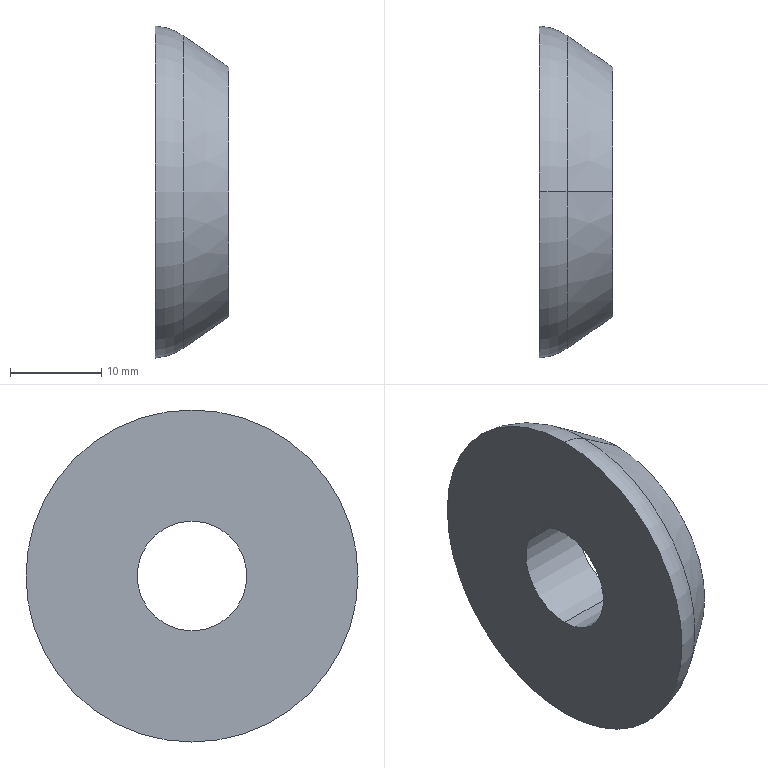Part | STEP file | Previa 01.sldasm-Part-13_Valor predeterminado | 1 solid | 8 faces | box 8 x 36.3 x 36.3 mm | volume 5808 mm3 | cylinder 2 | torus 2 | cone 2 | plane 2 | commonest cylinder face diameters 12 x2
STEP:
#1=CARTESIAN_POINT('',(0.,0.,0.));
#2=DIRECTION('',(0.,0.,1.));
#3=DIRECTION('',(1.,0.,0.));
#4=AXIS2_PLACEMENT_3D('',#1,#2,#3);
#5=CARTESIAN_POINT('',(72.6,0.,-6.));
#6=VERTEX_POINT('',#5);
#7=CARTESIAN_POINT('',(80.6,0.,-6.));
#8=VERTEX_POINT('',#7);
#9=CARTESIAN_POINT('',(55.897,0.,-6.));
#10=DIRECTION('',(1.,0.,0.));
#11=VECTOR('',#10,1.);
#12=LINE('',#9,#11);
#13=CARTESIAN_POINT('',(55.897,0.,0.));
#14=DIRECTION('',(1.,0.,0.));
#15=DIRECTION('',(0.,0.,-1.));
#16=AXIS2_PLACEMENT_3D('',#13,#14,#15);
#17=CYLINDRICAL_SURFACE('',#16,6.);
#18=CARTESIAN_POINT('',(6.283,0.));
#19=DIRECTION('',(0.,1.));
#20=VECTOR('',#19,1.);
#21=LINE('',#18,#20);
#22=(GEOMETRIC_REPRESENTATION_CONTEXT(2)PARAMETRIC_REPRESENTATION_CONTEXT()REPRESENTATION_CONTEXT('',''));
#23=DEFINITIONAL_REPRESENTATION('',(#21),#22);
#24=PCURVE('',#17,#23);
#25=CARTESIAN_POINT('',(55.897,0.,0.));
#26=DIRECTION('',(1.,0.,0.));
#27=DIRECTION('',(0.,0.,-1.));
#28=AXIS2_PLACEMENT_3D('',#25,#26,#27);
#29=CYLINDRICAL_SURFACE('',#28,6.);
#30=CARTESIAN_POINT('',(0.,0.));
#31=DIRECTION('',(0.,1.));
#32=VECTOR('',#31,1.);
#33=LINE('',#30,#32);
#34=(GEOMETRIC_REPRESENTATION_CONTEXT(2)PARAMETRIC_REPRESENTATION_CONTEXT()REPRESENTATION_CONTEXT('',''));
#35=DEFINITIONAL_REPRESENTATION('',(#33),#34);
#36=PCURVE('',#29,#35);
#37=SURFACE_CURVE('',#12,(#24,#36),.PCURVE_S1.);
#38=EDGE_CURVE('',#6,#8,#37,.T.);
#39=ORIENTED_EDGE('',*,*,#38,.T.);
#40=CARTESIAN_POINT('',(80.6,0.,6.));
#41=VERTEX_POINT('',#40);
#42=CARTESIAN_POINT('',(80.6,0.,0.));
#43=DIRECTION('',(-1.,0.,0.));
#44=DIRECTION('',(0.,0.,1.));
#45=AXIS2_PLACEMENT_3D('',#42,#43,#44);
#46=CIRCLE('',#45,6.);
#47=CARTESIAN_POINT('',(9.425,24.703));
#48=DIRECTION('',(-1.,0.));
#49=VECTOR('',#48,1.);
#50=LINE('',#47,#49);
#51=(GEOMETRIC_REPRESENTATION_CONTEXT(2)PARAMETRIC_REPRESENTATION_CONTEXT()REPRESENTATION_CONTEXT('',''));
#52=DEFINITIONAL_REPRESENTATION('',(#50),#51);
#53=PCURVE('',#17,#52);
#54=CARTESIAN_POINT('',(80.6,0.,0.));
#55=DIRECTION('',(-1.,0.,0.));
#56=DIRECTION('',(0.,0.,1.));
#57=AXIS2_PLACEMENT_3D('',#54,#55,#56);
#58=PLANE('',#57);
#59=CARTESIAN_POINT('',(0.,0.));
#60=DIRECTION('',(1.,0.));
#61=AXIS2_PLACEMENT_2D('',#59,#60);
#62=CIRCLE('',#61,6.);
#63=(GEOMETRIC_REPRESENTATION_CONTEXT(2)PARAMETRIC_REPRESENTATION_CONTEXT()REPRESENTATION_CONTEXT('',''));
#64=DEFINITIONAL_REPRESENTATION('',(#62),#63);
#65=PCURVE('',#58,#64);
#66=SURFACE_CURVE('',#46,(#53,#65),.PCURVE_S1.);
#67=EDGE_CURVE('',#8,#41,#66,.T.);
#68=ORIENTED_EDGE('',*,*,#67,.T.);
#69=CARTESIAN_POINT('',(72.6,0.,6.));
#70=VERTEX_POINT('',#69);
#71=CARTESIAN_POINT('',(55.897,0.,6.));
#72=DIRECTION('',(1.,0.,0.));
#73=VECTOR('',#72,1.);
#74=LINE('',#71,#73);
#75=CARTESIAN_POINT('',(3.142,0.));
#76=DIRECTION('',(0.,1.));
#77=VECTOR('',#76,1.);
#78=LINE('',#75,#77);
#79=(GEOMETRIC_REPRESENTATION_CONTEXT(2)PARAMETRIC_REPRESENTATION_CONTEXT()REPRESENTATION_CONTEXT('',''));
#80=DEFINITIONAL_REPRESENTATION('',(#78),#79);
#81=PCURVE('',#17,#80);
#82=CARTESIAN_POINT('',(3.142,0.));
#83=DIRECTION('',(0.,1.));
#84=VECTOR('',#83,1.);
#85=LINE('',#82,#84);
#86=(GEOMETRIC_REPRESENTATION_CONTEXT(2)PARAMETRIC_REPRESENTATION_CONTEXT()REPRESENTATION_CONTEXT('',''));
#87=DEFINITIONAL_REPRESENTATION('',(#85),#86);
#88=PCURVE('',#29,#87);
#89=SURFACE_CURVE('',#74,(#81,#88),.PCURVE_S1.);
#90=EDGE_CURVE('',#70,#41,#89,.T.);
#91=ORIENTED_EDGE('',*,*,#90,.F.);
#92=CARTESIAN_POINT('',(72.6,0.,0.));
#93=DIRECTION('',(-1.,0.,0.));
#94=DIRECTION('',(0.,0.,1.));
#95=AXIS2_PLACEMENT_3D('',#92,#93,#94);
#96=CIRCLE('',#95,6.);
#97=CARTESIAN_POINT('',(9.425,16.703));
#98=DIRECTION('',(-1.,0.));
#99=VECTOR('',#98,1.);
#100=LINE('',#97,#99);
#101=(GEOMETRIC_REPRESENTATION_CONTEXT(2)PARAMETRIC_REPRESENTATION_CONTEXT()REPRESENTATION_CONTEXT('',''));
#102=DEFINITIONAL_REPRESENTATION('',(#100),#101);
#103=PCURVE('',#17,#102);
#104=CARTESIAN_POINT('',(72.6,0.,0.));
#105=DIRECTION('',(-1.,0.,0.));
#106=DIRECTION('',(0.,0.,1.));
#107=AXIS2_PLACEMENT_3D('',#104,#105,#106);
#108=PLANE('',#107);
#109=CARTESIAN_POINT('',(0.,0.));
#110=DIRECTION('',(1.,0.));
#111=AXIS2_PLACEMENT_2D('',#109,#110);
#112=CIRCLE('',#111,6.);
#113=(GEOMETRIC_REPRESENTATION_CONTEXT(2)PARAMETRIC_REPRESENTATION_CONTEXT()REPRESENTATION_CONTEXT('',''));
#114=DEFINITIONAL_REPRESENTATION('',(#112),#113);
#115=PCURVE('',#108,#114);
#116=SURFACE_CURVE('',#96,(#103,#115),.PCURVE_S1.);
#117=EDGE_CURVE('',#6,#70,#116,.T.);
#118=ORIENTED_EDGE('',*,*,#117,.F.);
#119=EDGE_LOOP('',(#39,#68,#91,#118));
#120=FACE_BOUND('',#119,.F.);
#121=ADVANCED_FACE('',(#120),#17,.F.);
#122=CARTESIAN_POINT('',(75.622,0.,-17.096));
#123=VERTEX_POINT('',#122);
#124=CARTESIAN_POINT('',(75.622,0.,17.096));
#125=VERTEX_POINT('',#124);
#126=CARTESIAN_POINT('',(75.622,0.,0.));
#127=DIRECTION('',(1.,0.,0.));
#128=DIRECTION('',(0.,0.,1.));
#129=AXIS2_PLACEMENT_3D('',#126,#127,#128);
#130=CIRCLE('',#129,17.096);
#131=CARTESIAN_POINT('',(72.207,0.,0.));
#132=DIRECTION('',(-1.,0.,0.));
#133=DIRECTION('',(0.,0.,1.));
#134=AXIS2_PLACEMENT_3D('',#131,#132,#133);
#135=TOROIDAL_SURFACE('',#134,12.163,6.);
#136=CARTESIAN_POINT('',(6.283,5.678));
#137=DIRECTION('',(-1.,0.));
#138=VECTOR('',#137,1.);
#139=LINE('',#136,#138);
#140=(GEOMETRIC_REPRESENTATION_CONTEXT(2)PARAMETRIC_REPRESENTATION_CONTEXT()REPRESENTATION_CONTEXT('',''));
#141=DEFINITIONAL_REPRESENTATION('',(#139),#140);
#142=PCURVE('',#135,#141);
#143=CARTESIAN_POINT('',(74.1,0.,0.));
#144=DIRECTION('',(-1.,0.,0.));
#145=DIRECTION('',(0.,0.,1.));
#146=AXIS2_PLACEMENT_3D('',#143,#144,#145);
#147=CONICAL_SURFACE('',#146,18.15,0.6055);
#148=CARTESIAN_POINT('',(6.283,-1.522));
#149=DIRECTION('',(-1.,0.));
#150=VECTOR('',#149,1.);
#151=LINE('',#148,#150);
#152=(GEOMETRIC_REPRESENTATION_CONTEXT(2)PARAMETRIC_REPRESENTATION_CONTEXT()REPRESENTATION_CONTEXT('',''));
#153=DEFINITIONAL_REPRESENTATION('',(#151),#152);
#154=PCURVE('',#147,#153);
#155=SURFACE_CURVE('',#130,(#142,#154),.PCURVE_S1.);
#156=EDGE_CURVE('',#123,#125,#155,.T.);
#157=ORIENTED_EDGE('',*,*,#156,.F.);
#158=CARTESIAN_POINT('',(72.6,0.,-18.15));
#159=VERTEX_POINT('',#158);
#160=CARTESIAN_POINT('',(72.207,0.,-12.163));
#161=DIRECTION('',(0.,1.,0.));
#162=DIRECTION('',(0.,0.,1.));
#163=AXIS2_PLACEMENT_3D('',#160,#161,#162);
#164=CIRCLE('',#163,6.);
#165=CARTESIAN_POINT('',(3.142,3.142));
#166=DIRECTION('',(0.,1.));
#167=VECTOR('',#166,1.);
#168=LINE('',#165,#167);
#169=(GEOMETRIC_REPRESENTATION_CONTEXT(2)PARAMETRIC_REPRESENTATION_CONTEXT()REPRESENTATION_CONTEXT('',''));
#170=DEFINITIONAL_REPRESENTATION('',(#168),#169);
#171=PCURVE('',#135,#170);
#172=CARTESIAN_POINT('',(72.207,0.,0.));
#173=DIRECTION('',(-1.,0.,0.));
#174=DIRECTION('',(0.,0.,1.));
#175=AXIS2_PLACEMENT_3D('',#172,#173,#174);
#176=TOROIDAL_SURFACE('',#175,12.163,6.);
#177=CARTESIAN_POINT('',(3.142,3.142));
#178=DIRECTION('',(0.,1.));
#179=VECTOR('',#178,1.);
#180=LINE('',#177,#179);
#181=(GEOMETRIC_REPRESENTATION_CONTEXT(2)PARAMETRIC_REPRESENTATION_CONTEXT()REPRESENTATION_CONTEXT('',''));
#182=DEFINITIONAL_REPRESENTATION('',(#180),#181);
#183=PCURVE('',#176,#182);
#184=SURFACE_CURVE('',#164,(#171,#183),.PCURVE_S1.);
#185=EDGE_CURVE('',#123,#159,#184,.T.);
#186=ORIENTED_EDGE('',*,*,#185,.T.);
#187=CARTESIAN_POINT('',(72.6,0.,18.15));
#188=VERTEX_POINT('',#187);
#189=CARTESIAN_POINT('',(72.6,0.,0.));
#190=DIRECTION('',(-1.,0.,0.));
#191=DIRECTION('',(0.,-0.902,0.4317));
#192=AXIS2_PLACEMENT_3D('',#189,#190,#191);
#193=CIRCLE('',#192,18.15);
#194=CARTESIAN_POINT('',(-1.124,6.218));
#195=DIRECTION('',(1.,0.));
#196=VECTOR('',#195,1.);
#197=LINE('',#194,#196);
#198=(GEOMETRIC_REPRESENTATION_CONTEXT(2)PARAMETRIC_REPRESENTATION_CONTEXT()REPRESENTATION_CONTEXT('',''));
#199=DEFINITIONAL_REPRESENTATION('',(#197),#198);
#200=PCURVE('',#135,#199);
#201=CARTESIAN_POINT('',(0.,0.));
#202=DIRECTION('',(0.4317,-0.902));
#203=AXIS2_PLACEMENT_2D('',#201,#202);
#204=CIRCLE('',#203,18.15);
#205=(GEOMETRIC_REPRESENTATION_CONTEXT(2)PARAMETRIC_REPRESENTATION_CONTEXT()REPRESENTATION_CONTEXT('',''));
#206=DEFINITIONAL_REPRESENTATION('',(#204),#205);
#207=PCURVE('',#108,#206);
#208=SURFACE_CURVE('',#193,(#200,#207),.PCURVE_S1.);
#209=EDGE_CURVE('',#188,#159,#208,.T.);
#210=ORIENTED_EDGE('',*,*,#209,.F.);
#211=CARTESIAN_POINT('',(72.207,0.,12.163));
#212=DIRECTION('',(0.,-1.,0.));
#213=DIRECTION('',(1.,0.,0.));
#214=AXIS2_PLACEMENT_3D('',#211,#212,#213);
#215=CIRCLE('',#214,6.);
#216=CARTESIAN_POINT('',(0.,4.712));
#217=DIRECTION('',(0.,1.));
#218=VECTOR('',#217,1.);
#219=LINE('',#216,#218);
#220=(GEOMETRIC_REPRESENTATION_CONTEXT(2)PARAMETRIC_REPRESENTATION_CONTEXT()REPRESENTATION_CONTEXT('',''));
#221=DEFINITIONAL_REPRESENTATION('',(#219),#220);
#222=PCURVE('',#135,#221);
#223=CARTESIAN_POINT('',(6.283,4.712));
#224=DIRECTION('',(0.,1.));
#225=VECTOR('',#224,1.);
#226=LINE('',#223,#225);
#227=(GEOMETRIC_REPRESENTATION_CONTEXT(2)PARAMETRIC_REPRESENTATION_CONTEXT()REPRESENTATION_CONTEXT('',''));
#228=DEFINITIONAL_REPRESENTATION('',(#226),#227);
#229=PCURVE('',#176,#228);
#230=SURFACE_CURVE('',#215,(#222,#229),.PCURVE_S1.);
#231=EDGE_CURVE('',#125,#188,#230,.T.);
#232=ORIENTED_EDGE('',*,*,#231,.F.);
#233=EDGE_LOOP('',(#157,#186,#210,#232));
#234=FACE_BOUND('',#233,.T.);
#235=ADVANCED_FACE('',(#234),#135,.T.);
#236=CARTESIAN_POINT('',(80.6,0.,-13.65));
#237=VERTEX_POINT('',#236);
#238=CARTESIAN_POINT('',(80.6,0.,13.65));
#239=VERTEX_POINT('',#238);
#240=CARTESIAN_POINT('',(80.6,0.,0.));
#241=DIRECTION('',(1.,0.,0.));
#242=DIRECTION('',(0.,0.,1.));
#243=AXIS2_PLACEMENT_3D('',#240,#241,#242);
#244=CIRCLE('',#243,13.65);
#245=CARTESIAN_POINT('',(6.283,-6.5));
#246=DIRECTION('',(-1.,0.));
#247=VECTOR('',#246,1.);
#248=LINE('',#245,#247);
#249=(GEOMETRIC_REPRESENTATION_CONTEXT(2)PARAMETRIC_REPRESENTATION_CONTEXT()REPRESENTATION_CONTEXT('',''));
#250=DEFINITIONAL_REPRESENTATION('',(#248),#249);
#251=PCURVE('',#147,#250);
#252=CARTESIAN_POINT('',(13.65,0.));
#253=CARTESIAN_POINT('',(13.65,-23.642));
#254=CARTESIAN_POINT('',(-6.825,-11.821));
#255=CARTESIAN_POINT('',(-27.3,0.));
#256=CARTESIAN_POINT('',(-6.825,11.821));
#257=CARTESIAN_POINT('',(13.65,23.642));
#258=CARTESIAN_POINT('',(13.65,0.));
#259=(BOUNDED_CURVE()B_SPLINE_CURVE(2,(#252,#253,#254,#255,#256,#257,#258),.UNSPECIFIED.,.T.,.F.)B_SPLINE_CURVE_WITH_KNOTS((1,2,2,2,2,1),(-2.094,0.,2.094,4.189,6.283,8.378),.UNSPECIFIED.)CURVE()GEOMETRIC_REPRESENTATION_ITEM()RATIONAL_B_SPLINE_CURVE((1.,0.5,1.,0.5,1.,0.5,1.))REPRESENTATION_ITEM(''));
#260=(GEOMETRIC_REPRESENTATION_CONTEXT(2)PARAMETRIC_REPRESENTATION_CONTEXT()REPRESENTATION_CONTEXT('',''));
#261=DEFINITIONAL_REPRESENTATION('',(#259),#260);
#262=PCURVE('',#58,#261);
#263=SURFACE_CURVE('',#244,(#251,#262),.PCURVE_S1.);
#264=EDGE_CURVE('',#237,#239,#263,.T.);
#265=ORIENTED_EDGE('',*,*,#264,.F.);
#266=CARTESIAN_POINT('',(74.1,0.,-18.15));
#267=DIRECTION('',(-0.8222,0.,-0.5692));
#268=VECTOR('',#267,1.);
#269=LINE('',#266,#268);
#270=CARTESIAN_POINT('',(3.142,0.));
#271=DIRECTION('',(0.,1.));
#272=VECTOR('',#271,1.);
#273=LINE('',#270,#272);
#274=(GEOMETRIC_REPRESENTATION_CONTEXT(2)PARAMETRIC_REPRESENTATION_CONTEXT()REPRESENTATION_CONTEXT('',''));
#275=DEFINITIONAL_REPRESENTATION('',(#273),#274);
#276=PCURVE('',#147,#275);
#277=CARTESIAN_POINT('',(74.1,0.,0.));
#278=DIRECTION('',(-1.,0.,0.));
#279=DIRECTION('',(0.,0.,1.));
#280=AXIS2_PLACEMENT_3D('',#277,#278,#279);
#281=CONICAL_SURFACE('',#280,18.15,0.6055);
#282=CARTESIAN_POINT('',(3.142,0.));
#283=DIRECTION('',(0.,1.));
#284=VECTOR('',#283,1.);
#285=LINE('',#282,#284);
#286=(GEOMETRIC_REPRESENTATION_CONTEXT(2)PARAMETRIC_REPRESENTATION_CONTEXT()REPRESENTATION_CONTEXT('',''));
#287=DEFINITIONAL_REPRESENTATION('',(#285),#286);
#288=PCURVE('',#281,#287);
#289=SURFACE_CURVE('',#269,(#276,#288),.PCURVE_S1.);
#290=EDGE_CURVE('',#237,#123,#289,.T.);
#291=ORIENTED_EDGE('',*,*,#290,.T.);
#292=ORIENTED_EDGE('',*,*,#156,.T.);
#293=CARTESIAN_POINT('',(74.1,0.,18.15));
#294=DIRECTION('',(-0.8222,0.,0.5692));
#295=VECTOR('',#294,1.);
#296=LINE('',#293,#295);
#297=CARTESIAN_POINT('',(0.,0.));
#298=DIRECTION('',(0.,1.));
#299=VECTOR('',#298,1.);
#300=LINE('',#297,#299);
#301=(GEOMETRIC_REPRESENTATION_CONTEXT(2)PARAMETRIC_REPRESENTATION_CONTEXT()REPRESENTATION_CONTEXT('',''));
#302=DEFINITIONAL_REPRESENTATION('',(#300),#301);
#303=PCURVE('',#147,#302);
#304=CARTESIAN_POINT('',(6.283,0.));
#305=DIRECTION('',(0.,1.));
#306=VECTOR('',#305,1.);
#307=LINE('',#304,#306);
#308=(GEOMETRIC_REPRESENTATION_CONTEXT(2)PARAMETRIC_REPRESENTATION_CONTEXT()REPRESENTATION_CONTEXT('',''));
#309=DEFINITIONAL_REPRESENTATION('',(#307),#308);
#310=PCURVE('',#281,#309);
#311=SURFACE_CURVE('',#296,(#303,#310),.PCURVE_S1.);
#312=EDGE_CURVE('',#239,#125,#311,.T.);
#313=ORIENTED_EDGE('',*,*,#312,.F.);
#314=EDGE_LOOP('',(#265,#291,#292,#313));
#315=FACE_BOUND('',#314,.T.);
#316=ADVANCED_FACE('',(#315),#147,.T.);
#317=ORIENTED_EDGE('',*,*,#67,.T.);
#318=CARTESIAN_POINT('',(80.6,0.,0.));
#319=DIRECTION('',(-1.,0.,0.));
#320=DIRECTION('',(0.,0.,1.));
#321=AXIS2_PLACEMENT_3D('',#318,#319,#320);
#322=CIRCLE('',#321,6.);
#323=CARTESIAN_POINT('',(0.,0.));
#324=DIRECTION('',(1.,0.));
#325=AXIS2_PLACEMENT_2D('',#323,#324);
#326=CIRCLE('',#325,6.);
#327=(GEOMETRIC_REPRESENTATION_CONTEXT(2)PARAMETRIC_REPRESENTATION_CONTEXT()REPRESENTATION_CONTEXT('',''));
#328=DEFINITIONAL_REPRESENTATION('',(#326),#327);
#329=PCURVE('',#58,#328);
#330=CARTESIAN_POINT('',(3.142,24.703));
#331=DIRECTION('',(-1.,0.));
#332=VECTOR('',#331,1.);
#333=LINE('',#330,#332);
#334=(GEOMETRIC_REPRESENTATION_CONTEXT(2)PARAMETRIC_REPRESENTATION_CONTEXT()REPRESENTATION_CONTEXT('',''));
#335=DEFINITIONAL_REPRESENTATION('',(#333),#334);
#336=PCURVE('',#29,#335);
#337=SURFACE_CURVE('',#322,(#329,#336),.PCURVE_S1.);
#338=EDGE_CURVE('',#41,#8,#337,.T.);
#339=ORIENTED_EDGE('',*,*,#338,.T.);
#340=EDGE_LOOP('',(#317,#339));
#341=FACE_BOUND('',#340,.T.);
#342=CARTESIAN_POINT('',(80.6,0.,0.));
#343=DIRECTION('',(1.,0.,0.));
#344=DIRECTION('',(0.,0.,1.));
#345=AXIS2_PLACEMENT_3D('',#342,#343,#344);
#346=CIRCLE('',#345,13.65);
#347=CARTESIAN_POINT('',(13.65,0.));
#348=CARTESIAN_POINT('',(13.65,-23.642));
#349=CARTESIAN_POINT('',(-6.825,-11.821));
#350=CARTESIAN_POINT('',(-27.3,0.));
#351=CARTESIAN_POINT('',(-6.825,11.821));
#352=CARTESIAN_POINT('',(13.65,23.642));
#353=CARTESIAN_POINT('',(13.65,0.));
#354=(BOUNDED_CURVE()B_SPLINE_CURVE(2,(#347,#348,#349,#350,#351,#352,#353),.UNSPECIFIED.,.T.,.F.)B_SPLINE_CURVE_WITH_KNOTS((1,2,2,2,2,1),(-2.094,0.,2.094,4.189,6.283,8.378),.UNSPECIFIED.)CURVE()GEOMETRIC_REPRESENTATION_ITEM()RATIONAL_B_SPLINE_CURVE((1.,0.5,1.,0.5,1.,0.5,1.))REPRESENTATION_ITEM(''));
#355=(GEOMETRIC_REPRESENTATION_CONTEXT(2)PARAMETRIC_REPRESENTATION_CONTEXT()REPRESENTATION_CONTEXT('',''));
#356=DEFINITIONAL_REPRESENTATION('',(#354),#355);
#357=PCURVE('',#58,#356);
#358=CARTESIAN_POINT('',(6.283,-6.5));
#359=DIRECTION('',(-1.,0.));
#360=VECTOR('',#359,1.);
#361=LINE('',#358,#360);
#362=(GEOMETRIC_REPRESENTATION_CONTEXT(2)PARAMETRIC_REPRESENTATION_CONTEXT()REPRESENTATION_CONTEXT('',''));
#363=DEFINITIONAL_REPRESENTATION('',(#361),#362);
#364=PCURVE('',#281,#363);
#365=SURFACE_CURVE('',#346,(#357,#364),.PCURVE_S1.);
#366=EDGE_CURVE('',#239,#237,#365,.T.);
#367=ORIENTED_EDGE('',*,*,#366,.T.);
#368=ORIENTED_EDGE('',*,*,#264,.T.);
#369=EDGE_LOOP('',(#367,#368));
#370=FACE_BOUND('',#369,.T.);
#371=ADVANCED_FACE('',(#341,#370),#58,.F.);
#372=ORIENTED_EDGE('',*,*,#117,.F.);
#373=CARTESIAN_POINT('',(72.6,0.,0.));
#374=DIRECTION('',(-1.,0.,0.));
#375=DIRECTION('',(0.,0.,1.));
#376=AXIS2_PLACEMENT_3D('',#373,#374,#375);
#377=CIRCLE('',#376,6.);
#378=CARTESIAN_POINT('',(0.,0.));
#379=DIRECTION('',(1.,0.));
#380=AXIS2_PLACEMENT_2D('',#378,#379);
#381=CIRCLE('',#380,6.);
#382=(GEOMETRIC_REPRESENTATION_CONTEXT(2)PARAMETRIC_REPRESENTATION_CONTEXT()REPRESENTATION_CONTEXT('',''));
#383=DEFINITIONAL_REPRESENTATION('',(#381),#382);
#384=PCURVE('',#108,#383);
#385=CARTESIAN_POINT('',(3.142,16.703));
#386=DIRECTION('',(-1.,0.));
#387=VECTOR('',#386,1.);
#388=LINE('',#385,#387);
#389=(GEOMETRIC_REPRESENTATION_CONTEXT(2)PARAMETRIC_REPRESENTATION_CONTEXT()REPRESENTATION_CONTEXT('',''));
#390=DEFINITIONAL_REPRESENTATION('',(#388),#389);
#391=PCURVE('',#29,#390);
#392=SURFACE_CURVE('',#377,(#384,#391),.PCURVE_S1.);
#393=EDGE_CURVE('',#70,#6,#392,.T.);
#394=ORIENTED_EDGE('',*,*,#393,.F.);
#395=EDGE_LOOP('',(#372,#394));
#396=FACE_BOUND('',#395,.T.);
#397=ORIENTED_EDGE('',*,*,#209,.T.);
#398=CARTESIAN_POINT('',(72.6,0.,0.));
#399=DIRECTION('',(-1.,0.,0.));
#400=DIRECTION('',(0.,-0.902,0.4317));
#401=AXIS2_PLACEMENT_3D('',#398,#399,#400);
#402=CIRCLE('',#401,18.15);
#403=CARTESIAN_POINT('',(0.,0.));
#404=DIRECTION('',(0.4317,-0.902));
#405=AXIS2_PLACEMENT_2D('',#403,#404);
#406=CIRCLE('',#405,18.15);
#407=(GEOMETRIC_REPRESENTATION_CONTEXT(2)PARAMETRIC_REPRESENTATION_CONTEXT()REPRESENTATION_CONTEXT('',''));
#408=DEFINITIONAL_REPRESENTATION('',(#406),#407);
#409=PCURVE('',#108,#408);
#410=CARTESIAN_POINT('',(-1.124,6.218));
#411=DIRECTION('',(1.,0.));
#412=VECTOR('',#411,1.);
#413=LINE('',#410,#412);
#414=(GEOMETRIC_REPRESENTATION_CONTEXT(2)PARAMETRIC_REPRESENTATION_CONTEXT()REPRESENTATION_CONTEXT('',''));
#415=DEFINITIONAL_REPRESENTATION('',(#413),#414);
#416=PCURVE('',#176,#415);
#417=SURFACE_CURVE('',#402,(#409,#416),.PCURVE_S1.);
#418=EDGE_CURVE('',#159,#188,#417,.T.);
#419=ORIENTED_EDGE('',*,*,#418,.T.);
#420=EDGE_LOOP('',(#397,#419));
#421=FACE_BOUND('',#420,.T.);
#422=ADVANCED_FACE('',(#396,#421),#108,.T.);
#423=ORIENTED_EDGE('',*,*,#290,.F.);
#424=ORIENTED_EDGE('',*,*,#366,.F.);
#425=ORIENTED_EDGE('',*,*,#312,.T.);
#426=CARTESIAN_POINT('',(75.622,0.,0.));
#427=DIRECTION('',(1.,0.,0.));
#428=DIRECTION('',(0.,0.,1.));
#429=AXIS2_PLACEMENT_3D('',#426,#427,#428);
#430=CIRCLE('',#429,17.096);
#431=CARTESIAN_POINT('',(6.283,-1.522));
#432=DIRECTION('',(-1.,0.));
#433=VECTOR('',#432,1.);
#434=LINE('',#431,#433);
#435=(GEOMETRIC_REPRESENTATION_CONTEXT(2)PARAMETRIC_REPRESENTATION_CONTEXT()REPRESENTATION_CONTEXT('',''));
#436=DEFINITIONAL_REPRESENTATION('',(#434),#435);
#437=PCURVE('',#281,#436);
#438=CARTESIAN_POINT('',(6.283,5.678));
#439=DIRECTION('',(-1.,0.));
#440=VECTOR('',#439,1.);
#441=LINE('',#438,#440);
#442=(GEOMETRIC_REPRESENTATION_CONTEXT(2)PARAMETRIC_REPRESENTATION_CONTEXT()REPRESENTATION_CONTEXT('',''));
#443=DEFINITIONAL_REPRESENTATION('',(#441),#442);
#444=PCURVE('',#176,#443);
#445=SURFACE_CURVE('',#430,(#437,#444),.PCURVE_S1.);
#446=EDGE_CURVE('',#125,#123,#445,.T.);
#447=ORIENTED_EDGE('',*,*,#446,.T.);
#448=EDGE_LOOP('',(#423,#424,#425,#447));
#449=FACE_BOUND('',#448,.T.);
#450=ADVANCED_FACE('',(#449),#281,.T.);
#451=ORIENTED_EDGE('',*,*,#185,.F.);
#452=ORIENTED_EDGE('',*,*,#446,.F.);
#453=ORIENTED_EDGE('',*,*,#231,.T.);
#454=ORIENTED_EDGE('',*,*,#418,.F.);
#455=EDGE_LOOP('',(#451,#452,#453,#454));
#456=FACE_BOUND('',#455,.T.);
#457=ADVANCED_FACE('',(#456),#176,.T.);
#458=ORIENTED_EDGE('',*,*,#338,.T.);
#459=ORIENTED_EDGE('',*,*,#38,.F.);
#460=ORIENTED_EDGE('',*,*,#393,.F.);
#461=ORIENTED_EDGE('',*,*,#90,.T.);
#462=EDGE_LOOP('',(#458,#459,#460,#461));
#463=FACE_BOUND('',#462,.F.);
#464=ADVANCED_FACE('',(#463),#29,.F.);
#465=CLOSED_SHELL('',(#121,#235,#316,#371,#422,#450,#457,#464));
#466=MANIFOLD_SOLID_BREP('',#465);
#467=(LENGTH_UNIT()NAMED_UNIT(*)SI_UNIT(.MILLI.,.METRE.));
#468=UNCERTAINTY_MEASURE_WITH_UNIT(LENGTH_MEASURE(0.0000001),#467,'','');
#469=(NAMED_UNIT(*)PLANE_ANGLE_UNIT()SI_UNIT($,.RADIAN.));
#470=(NAMED_UNIT(*)SI_UNIT($,.STERADIAN.)SOLID_ANGLE_UNIT());
#471=(GEOMETRIC_REPRESENTATION_CONTEXT(3)GLOBAL_UNCERTAINTY_ASSIGNED_CONTEXT((#468))GLOBAL_UNIT_ASSIGNED_CONTEXT((#467,#469,#470))REPRESENTATION_CONTEXT('',''));
#472=ADVANCED_BREP_SHAPE_REPRESENTATION('',(#4,#466),#471);